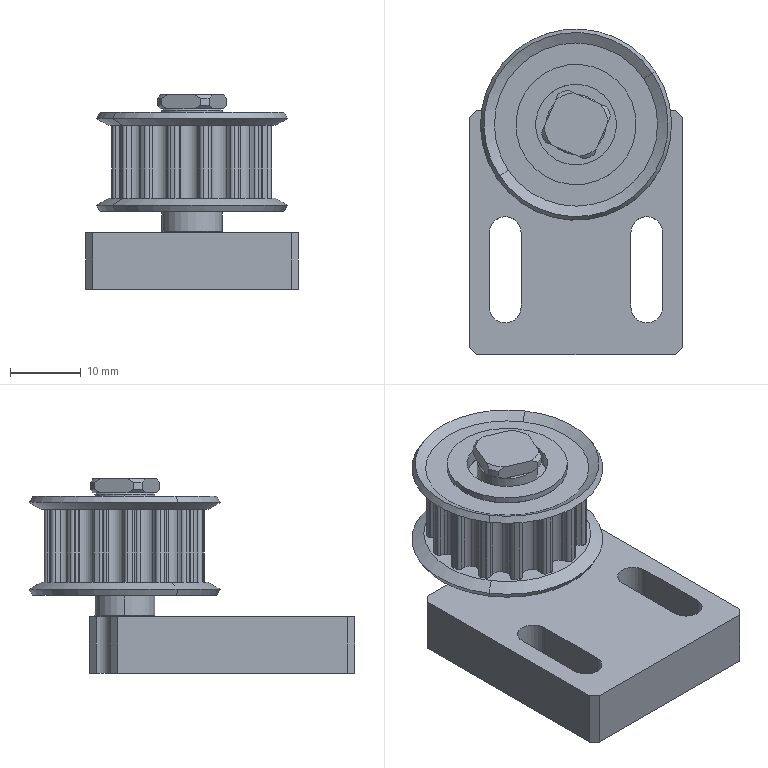Part | NX | features BREP 6 | 7 solids | 285 faces | box 30 x 46 x 27.5 mm | volume 12594 mm3 | cylinder 156 | plane 55 | cone 42 | torus 32 | commonest cylinder face diameters 1.02 x38 5.08 x31 2.74 x20 22.73 x15 6 x8 13 x8